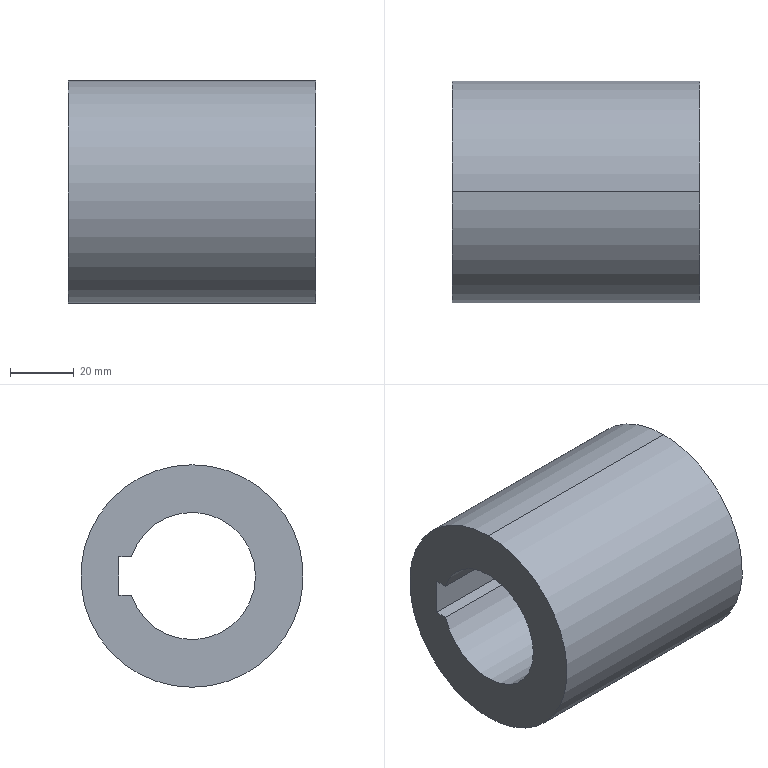Part | STEP file | Produce dryer double-row sprocket | 1 solid | 8 faces | box 78 x 70 x 70 mm | volume 199069 mm3 | plane 5 | cylinder 3 | commonest cylinder face diameters 70 x2 40 x1
STEP:
#1=CARTESIAN_POINT('',(-69.5,0.,-35.));
#2=VERTEX_POINT('',#1);
#3=CARTESIAN_POINT('',(-69.5,0.,35.));
#4=VERTEX_POINT('',#3);
#5=CARTESIAN_POINT('',(-69.5,0.,0.));
#6=DIRECTION('',(1.,0.,0.));
#7=DIRECTION('',(0.,0.,-1.));
#8=AXIS2_PLACEMENT_3D('',#5,#6,#7);
#9=CIRCLE('',#8,35.);
#10=EDGE_CURVE('',#2,#4,#9,.T.);
#11=ORIENTED_EDGE('',*,*,#10,.T.);
#12=CARTESIAN_POINT('',(8.5,0.,35.));
#13=VERTEX_POINT('',#12);
#14=CARTESIAN_POINT('',(0.,0.,35.));
#15=DIRECTION('',(1.,0.,0.));
#16=VECTOR('',#15,1000.);
#17=LINE('',#14,#16);
#18=EDGE_CURVE('',#4,#13,#17,.T.);
#19=ORIENTED_EDGE('',*,*,#18,.T.);
#20=CARTESIAN_POINT('',(8.5,0.,-35.));
#21=VERTEX_POINT('',#20);
#22=CARTESIAN_POINT('',(8.5,0.,0.));
#23=DIRECTION('',(1.,0.,0.));
#24=DIRECTION('',(0.,0.,-1.));
#25=AXIS2_PLACEMENT_3D('',#22,#23,#24);
#26=CIRCLE('',#25,35.);
#27=EDGE_CURVE('',#21,#13,#26,.T.);
#28=ORIENTED_EDGE('',*,*,#27,.F.);
#29=CARTESIAN_POINT('',(0.,0.,-35.));
#30=DIRECTION('',(1.,0.,0.));
#31=VECTOR('',#30,1000.);
#32=LINE('',#29,#31);
#33=EDGE_CURVE('',#2,#21,#32,.T.);
#34=ORIENTED_EDGE('',*,*,#33,.F.);
#35=EDGE_LOOP('',(#11,#19,#28,#34));
#36=FACE_OUTER_BOUND('',#35,.T.);
#37=CARTESIAN_POINT('',(0.,0.,0.));
#38=DIRECTION('',(1.,0.,0.));
#39=DIRECTION('',(0.,0.,-1.));
#40=AXIS2_PLACEMENT_3D('',#37,#38,#39);
#41=CYLINDRICAL_SURFACE('',#40,35.);
#42=ADVANCED_FACE('',(#36),#41,.T.);
#43=CARTESIAN_POINT('',(-69.5,19.079,-6.));
#44=VERTEX_POINT('',#43);
#45=CARTESIAN_POINT('',(-69.5,23.,-6.));
#46=VERTEX_POINT('',#45);
#47=CARTESIAN_POINT('',(-69.5,23.,-6.));
#48=DIRECTION('',(0.,1.,0.));
#49=VECTOR('',#48,1000.);
#50=LINE('',#47,#49);
#51=EDGE_CURVE('',#44,#46,#50,.T.);
#52=ORIENTED_EDGE('',*,*,#51,.T.);
#53=CARTESIAN_POINT('',(-69.5,23.,6.));
#54=VERTEX_POINT('',#53);
#55=CARTESIAN_POINT('',(-69.5,23.,6.));
#56=DIRECTION('',(0.,0.,1.));
#57=VECTOR('',#56,1000.);
#58=LINE('',#55,#57);
#59=EDGE_CURVE('',#46,#54,#58,.T.);
#60=ORIENTED_EDGE('',*,*,#59,.T.);
#61=CARTESIAN_POINT('',(-69.5,19.079,6.));
#62=VERTEX_POINT('',#61);
#63=CARTESIAN_POINT('',(-69.5,23.,6.));
#64=DIRECTION('',(0.,-1.,0.));
#65=VECTOR('',#64,1000.);
#66=LINE('',#63,#65);
#67=EDGE_CURVE('',#54,#62,#66,.T.);
#68=ORIENTED_EDGE('',*,*,#67,.T.);
#69=CARTESIAN_POINT('',(-69.5,0.,0.));
#70=DIRECTION('',(1.,0.,0.));
#71=DIRECTION('',(0.,1.,0.));
#72=AXIS2_PLACEMENT_3D('',#69,#70,#71);
#73=CIRCLE('',#72,20.);
#74=EDGE_CURVE('',#62,#44,#73,.T.);
#75=ORIENTED_EDGE('',*,*,#74,.T.);
#76=EDGE_LOOP('',(#52,#60,#68,#75));
#77=FACE_BOUND('',#76,.T.);
#78=ORIENTED_EDGE('',*,*,#10,.F.);
#79=CARTESIAN_POINT('',(-69.5,0.,0.));
#80=DIRECTION('',(1.,0.,0.));
#81=DIRECTION('',(0.,0.,-1.));
#82=AXIS2_PLACEMENT_3D('',#79,#80,#81);
#83=CIRCLE('',#82,35.);
#84=EDGE_CURVE('',#4,#2,#83,.T.);
#85=ORIENTED_EDGE('',*,*,#84,.F.);
#86=EDGE_LOOP('',(#78,#85));
#87=FACE_OUTER_BOUND('',#86,.T.);
#88=CARTESIAN_POINT('',(-69.5,0.,0.));
#89=DIRECTION('',(-1.,0.,0.));
#90=DIRECTION('',(0.,0.,1.));
#91=AXIS2_PLACEMENT_3D('',#88,#89,#90);
#92=PLANE('',#91);
#93=ADVANCED_FACE('',(#77,#87),#92,.T.);
#94=ORIENTED_EDGE('',*,*,#18,.F.);
#95=ORIENTED_EDGE('',*,*,#84,.T.);
#96=ORIENTED_EDGE('',*,*,#33,.T.);
#97=CARTESIAN_POINT('',(8.5,0.,0.));
#98=DIRECTION('',(1.,0.,0.));
#99=DIRECTION('',(0.,0.,-1.));
#100=AXIS2_PLACEMENT_3D('',#97,#98,#99);
#101=CIRCLE('',#100,35.);
#102=EDGE_CURVE('',#13,#21,#101,.T.);
#103=ORIENTED_EDGE('',*,*,#102,.F.);
#104=EDGE_LOOP('',(#94,#95,#96,#103));
#105=FACE_OUTER_BOUND('',#104,.T.);
#106=CARTESIAN_POINT('',(0.,0.,0.));
#107=DIRECTION('',(1.,0.,0.));
#108=DIRECTION('',(0.,0.,-1.));
#109=AXIS2_PLACEMENT_3D('',#106,#107,#108);
#110=CYLINDRICAL_SURFACE('',#109,35.);
#111=ADVANCED_FACE('',(#105),#110,.T.);
#112=CARTESIAN_POINT('',(8.5,19.079,-6.));
#113=VERTEX_POINT('',#112);
#114=CARTESIAN_POINT('',(8.5,23.,-6.));
#115=VERTEX_POINT('',#114);
#116=CARTESIAN_POINT('',(8.5,23.,-6.));
#117=DIRECTION('',(0.,1.,0.));
#118=VECTOR('',#117,1000.);
#119=LINE('',#116,#118);
#120=EDGE_CURVE('',#113,#115,#119,.T.);
#121=ORIENTED_EDGE('',*,*,#120,.F.);
#122=CARTESIAN_POINT('',(8.5,19.079,6.));
#123=VERTEX_POINT('',#122);
#124=CARTESIAN_POINT('',(8.5,0.,0.));
#125=DIRECTION('',(1.,0.,0.));
#126=DIRECTION('',(0.,1.,0.));
#127=AXIS2_PLACEMENT_3D('',#124,#125,#126);
#128=CIRCLE('',#127,20.);
#129=EDGE_CURVE('',#123,#113,#128,.T.);
#130=ORIENTED_EDGE('',*,*,#129,.F.);
#131=CARTESIAN_POINT('',(8.5,23.,6.));
#132=VERTEX_POINT('',#131);
#133=CARTESIAN_POINT('',(8.5,23.,6.));
#134=DIRECTION('',(0.,-1.,0.));
#135=VECTOR('',#134,1000.);
#136=LINE('',#133,#135);
#137=EDGE_CURVE('',#132,#123,#136,.T.);
#138=ORIENTED_EDGE('',*,*,#137,.F.);
#139=CARTESIAN_POINT('',(8.5,23.,6.));
#140=DIRECTION('',(0.,0.,1.));
#141=VECTOR('',#140,1000.);
#142=LINE('',#139,#141);
#143=EDGE_CURVE('',#115,#132,#142,.T.);
#144=ORIENTED_EDGE('',*,*,#143,.F.);
#145=EDGE_LOOP('',(#121,#130,#138,#144));
#146=FACE_BOUND('',#145,.T.);
#147=ORIENTED_EDGE('',*,*,#27,.T.);
#148=ORIENTED_EDGE('',*,*,#102,.T.);
#149=EDGE_LOOP('',(#147,#148));
#150=FACE_OUTER_BOUND('',#149,.T.);
#151=CARTESIAN_POINT('',(8.5,35.,0.));
#152=DIRECTION('',(1.,0.,0.));
#153=DIRECTION('',(0.,0.,-1.));
#154=AXIS2_PLACEMENT_3D('',#151,#152,#153);
#155=PLANE('',#154);
#156=ADVANCED_FACE('',(#146,#150),#155,.T.);
#157=ORIENTED_EDGE('',*,*,#129,.T.);
#158=CARTESIAN_POINT('',(-69.5,19.079,-6.));
#159=DIRECTION('',(-1.,0.,0.));
#160=VECTOR('',#159,1000.);
#161=LINE('',#158,#160);
#162=EDGE_CURVE('',#113,#44,#161,.T.);
#163=ORIENTED_EDGE('',*,*,#162,.T.);
#164=ORIENTED_EDGE('',*,*,#74,.F.);
#165=CARTESIAN_POINT('',(-69.5,19.079,6.));
#166=DIRECTION('',(1.,0.,0.));
#167=VECTOR('',#166,1000.);
#168=LINE('',#165,#167);
#169=EDGE_CURVE('',#62,#123,#168,.T.);
#170=ORIENTED_EDGE('',*,*,#169,.T.);
#171=EDGE_LOOP('',(#157,#163,#164,#170));
#172=FACE_OUTER_BOUND('',#171,.T.);
#173=CARTESIAN_POINT('',(-69.5,0.,0.));
#174=DIRECTION('',(1.,0.,0.));
#175=DIRECTION('',(0.,1.,0.));
#176=AXIS2_PLACEMENT_3D('',#173,#174,#175);
#177=CYLINDRICAL_SURFACE('',#176,20.);
#178=ADVANCED_FACE('',(#172),#177,.F.);
#179=ORIENTED_EDGE('',*,*,#120,.T.);
#180=CARTESIAN_POINT('',(-69.5,23.,-6.));
#181=DIRECTION('',(1.,0.,0.));
#182=VECTOR('',#181,1000.);
#183=LINE('',#180,#182);
#184=EDGE_CURVE('',#46,#115,#183,.T.);
#185=ORIENTED_EDGE('',*,*,#184,.F.);
#186=ORIENTED_EDGE('',*,*,#51,.F.);
#187=ORIENTED_EDGE('',*,*,#162,.F.);
#188=EDGE_LOOP('',(#179,#185,#186,#187));
#189=FACE_OUTER_BOUND('',#188,.T.);
#190=CARTESIAN_POINT('',(-69.5,23.,-6.));
#191=DIRECTION('',(0.,0.,-1.));
#192=DIRECTION('',(0.,1.,0.));
#193=AXIS2_PLACEMENT_3D('',#190,#191,#192);
#194=PLANE('',#193);
#195=ADVANCED_FACE('',(#189),#194,.F.);
#196=ORIENTED_EDGE('',*,*,#67,.F.);
#197=CARTESIAN_POINT('',(-69.5,23.,6.));
#198=DIRECTION('',(1.,0.,0.));
#199=VECTOR('',#198,1000.);
#200=LINE('',#197,#199);
#201=EDGE_CURVE('',#54,#132,#200,.T.);
#202=ORIENTED_EDGE('',*,*,#201,.T.);
#203=ORIENTED_EDGE('',*,*,#137,.T.);
#204=ORIENTED_EDGE('',*,*,#169,.F.);
#205=EDGE_LOOP('',(#196,#202,#203,#204));
#206=FACE_OUTER_BOUND('',#205,.T.);
#207=CARTESIAN_POINT('',(-69.5,23.,6.));
#208=DIRECTION('',(0.,0.,1.));
#209=DIRECTION('',(1.,0.,0.));
#210=AXIS2_PLACEMENT_3D('',#207,#208,#209);
#211=PLANE('',#210);
#212=ADVANCED_FACE('',(#206),#211,.F.);
#213=ORIENTED_EDGE('',*,*,#143,.T.);
#214=ORIENTED_EDGE('',*,*,#201,.F.);
#215=ORIENTED_EDGE('',*,*,#59,.F.);
#216=ORIENTED_EDGE('',*,*,#184,.T.);
#217=EDGE_LOOP('',(#213,#214,#215,#216));
#218=FACE_OUTER_BOUND('',#217,.T.);
#219=CARTESIAN_POINT('',(-69.5,23.,6.));
#220=DIRECTION('',(0.,1.,0.));
#221=DIRECTION('',(0.,0.,1.));
#222=AXIS2_PLACEMENT_3D('',#219,#220,#221);
#223=PLANE('',#222);
#224=ADVANCED_FACE('',(#218),#223,.F.);
#225=CLOSED_SHELL('',(#42,#93,#111,#156,#178,#195,#212,#224));
#226=MANIFOLD_SOLID_BREP('',#225);
#227=CARTESIAN_POINT('',(0.,0.,0.));
#228=DIRECTION('',(0.,0.,1.));
#229=DIRECTION('',(1.,0.,0.));
#230=AXIS2_PLACEMENT_3D('',#227,#228,#229);
#231=(LENGTH_UNIT()NAMED_UNIT(*)SI_UNIT(.MILLI.,.METRE.));
#232=UNCERTAINTY_MEASURE_WITH_UNIT(LENGTH_MEASURE(0.00001),#231,'','');
#233=(NAMED_UNIT(*)PLANE_ANGLE_UNIT()SI_UNIT($,.RADIAN.));
#234=(NAMED_UNIT(*)SI_UNIT($,.STERADIAN.)SOLID_ANGLE_UNIT());
#235=(GEOMETRIC_REPRESENTATION_CONTEXT(3)GLOBAL_UNCERTAINTY_ASSIGNED_CONTEXT((#232))GLOBAL_UNIT_ASSIGNED_CONTEXT((#231,#233,#234))REPRESENTATION_CONTEXT('',''));
#236=ADVANCED_BREP_SHAPE_REPRESENTATION('',(#226,#230),#235);